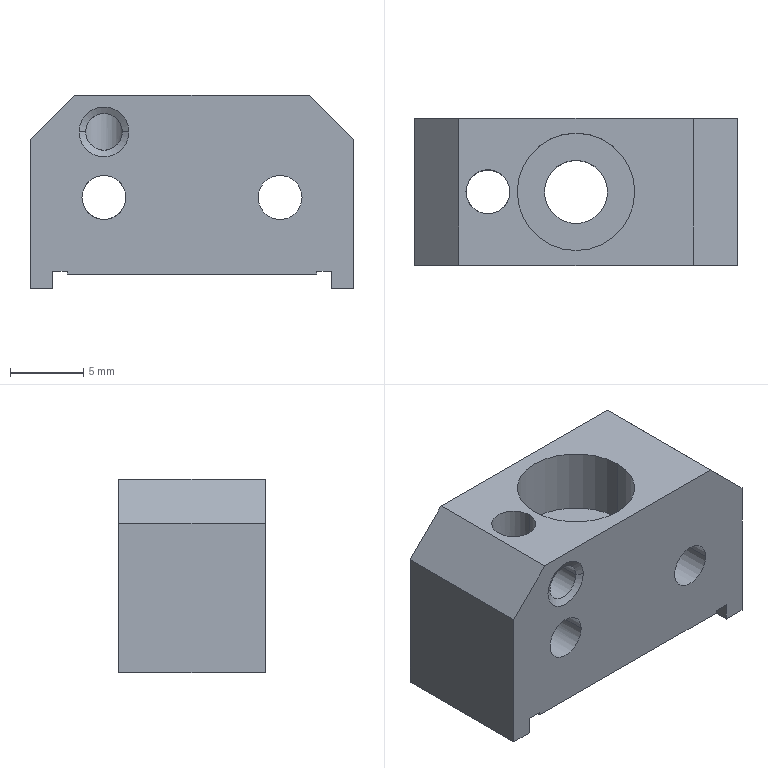Part | NX | 1 solid | 35 faces | box 22 x 10 x 13.2 mm | volume 2054 mm3 | plane 17 | cylinder 16 | cone 2 | commonest cylinder face diameters 3 x10 2.5 x2 4.3 x2 8 x2
STEP:
#1=CARTESIAN_POINT('',(9.5,5.,-6.6));
#2=VERTEX_POINT('',#1);
#3=CARTESIAN_POINT('',(9.5,-5.,-6.6));
#4=VERTEX_POINT('',#3);
#5=CARTESIAN_POINT('',(9.5,5.,-6.6));
#6=DIRECTION('',(0.,-1.,0.));
#7=VECTOR('',#6,1000.);
#8=LINE('',#5,#7);
#9=EDGE_CURVE('',#2,#4,#8,.T.);
#10=ORIENTED_EDGE('',*,*,#9,.F.);
#11=CARTESIAN_POINT('',(11.,5.,-6.6));
#12=VERTEX_POINT('',#11);
#13=CARTESIAN_POINT('',(0.,5.,-6.6));
#14=DIRECTION('',(-1.,0.,0.));
#15=VECTOR('',#14,1000.);
#16=LINE('',#13,#15);
#17=EDGE_CURVE('',#12,#2,#16,.T.);
#18=ORIENTED_EDGE('',*,*,#17,.F.);
#19=CARTESIAN_POINT('',(11.,-5.,-6.6));
#20=VERTEX_POINT('',#19);
#21=CARTESIAN_POINT('',(11.,5.,-6.6));
#22=DIRECTION('',(0.,-1.,0.));
#23=VECTOR('',#22,1000.);
#24=LINE('',#21,#23);
#25=EDGE_CURVE('',#12,#20,#24,.T.);
#26=ORIENTED_EDGE('',*,*,#25,.T.);
#27=CARTESIAN_POINT('',(0.,-5.,-6.6));
#28=DIRECTION('',(1.,0.,0.));
#29=VECTOR('',#28,1000.);
#30=LINE('',#27,#29);
#31=EDGE_CURVE('',#4,#20,#30,.T.);
#32=ORIENTED_EDGE('',*,*,#31,.F.);
#33=EDGE_LOOP('',(#10,#18,#26,#32));
#34=FACE_BOUND('',#33,.T.);
#35=CARTESIAN_POINT('',(0.,0.,-6.6));
#36=DIRECTION('',(0.,0.,1.));
#37=DIRECTION('',(1.,0.,0.));
#38=AXIS2_PLACEMENT_3D('',#35,#36,#37);
#39=PLANE('',#38);
#40=ADVANCED_FACE('',(#34),#39,.F.);
#41=CARTESIAN_POINT('',(9.5,5.,-5.4));
#42=VERTEX_POINT('',#41);
#43=CARTESIAN_POINT('',(9.5,5.,0.));
#44=DIRECTION('',(0.,0.,1.));
#45=VECTOR('',#44,1000.);
#46=LINE('',#43,#45);
#47=EDGE_CURVE('',#2,#42,#46,.T.);
#48=ORIENTED_EDGE('',*,*,#47,.F.);
#49=ORIENTED_EDGE('',*,*,#9,.T.);
#50=CARTESIAN_POINT('',(9.5,-5.,-5.4));
#51=VERTEX_POINT('',#50);
#52=CARTESIAN_POINT('',(9.5,-5.,0.));
#53=DIRECTION('',(0.,0.,-1.));
#54=VECTOR('',#53,1000.);
#55=LINE('',#52,#54);
#56=EDGE_CURVE('',#51,#4,#55,.T.);
#57=ORIENTED_EDGE('',*,*,#56,.F.);
#58=CARTESIAN_POINT('',(9.5,5.,-5.4));
#59=DIRECTION('',(0.,-1.,0.));
#60=VECTOR('',#59,1000.);
#61=LINE('',#58,#60);
#62=EDGE_CURVE('',#42,#51,#61,.T.);
#63=ORIENTED_EDGE('',*,*,#62,.F.);
#64=EDGE_LOOP('',(#48,#49,#57,#63));
#65=FACE_BOUND('',#64,.T.);
#66=CARTESIAN_POINT('',(9.5,-5.,-6.6));
#67=DIRECTION('',(1.,0.,0.));
#68=DIRECTION('',(0.,1.,0.));
#69=AXIS2_PLACEMENT_3D('',#66,#67,#68);
#70=PLANE('',#69);
#71=ADVANCED_FACE('',(#65),#70,.F.);
#72=CARTESIAN_POINT('',(-8.5,5.,-5.6));
#73=VERTEX_POINT('',#72);
#74=CARTESIAN_POINT('',(-8.5,5.,-5.4));
#75=VERTEX_POINT('',#74);
#76=CARTESIAN_POINT('',(-8.5,5.,0.));
#77=DIRECTION('',(0.,0.,1.));
#78=VECTOR('',#77,1000.);
#79=LINE('',#76,#78);
#80=EDGE_CURVE('',#73,#75,#79,.T.);
#81=ORIENTED_EDGE('',*,*,#80,.T.);
#82=CARTESIAN_POINT('',(-9.5,5.,-5.4));
#83=VERTEX_POINT('',#82);
#84=CARTESIAN_POINT('',(0.,5.,-5.4));
#85=DIRECTION('',(-1.,0.,0.));
#86=VECTOR('',#85,1000.);
#87=LINE('',#84,#86);
#88=EDGE_CURVE('',#75,#83,#87,.T.);
#89=ORIENTED_EDGE('',*,*,#88,.T.);
#90=CARTESIAN_POINT('',(-9.5,5.,-6.6));
#91=VERTEX_POINT('',#90);
#92=CARTESIAN_POINT('',(-9.5,5.,0.));
#93=DIRECTION('',(0.,0.,-1.));
#94=VECTOR('',#93,1000.);
#95=LINE('',#92,#94);
#96=EDGE_CURVE('',#83,#91,#95,.T.);
#97=ORIENTED_EDGE('',*,*,#96,.T.);
#98=CARTESIAN_POINT('',(-11.,5.,-6.6));
#99=VERTEX_POINT('',#98);
#100=CARTESIAN_POINT('',(0.,5.,-6.6));
#101=DIRECTION('',(-1.,0.,0.));
#102=VECTOR('',#101,1000.);
#103=LINE('',#100,#102);
#104=EDGE_CURVE('',#91,#99,#103,.T.);
#105=ORIENTED_EDGE('',*,*,#104,.T.);
#106=CARTESIAN_POINT('',(-11.,5.,3.6));
#107=VERTEX_POINT('',#106);
#108=CARTESIAN_POINT('',(-11.,5.,0.));
#109=DIRECTION('',(0.,0.,-1.));
#110=VECTOR('',#109,1000.);
#111=LINE('',#108,#110);
#112=EDGE_CURVE('',#107,#99,#111,.T.);
#113=ORIENTED_EDGE('',*,*,#112,.F.);
#114=CARTESIAN_POINT('',(-8.,5.,6.6));
#115=VERTEX_POINT('',#114);
#116=CARTESIAN_POINT('',(-14.6,5.,0.));
#117=DIRECTION('',(0.7071,0.,0.7071));
#118=VECTOR('',#117,1000.);
#119=LINE('',#116,#118);
#120=EDGE_CURVE('',#107,#115,#119,.T.);
#121=ORIENTED_EDGE('',*,*,#120,.T.);
#122=CARTESIAN_POINT('',(8.,5.,6.6));
#123=VERTEX_POINT('',#122);
#124=CARTESIAN_POINT('',(0.,5.,6.6));
#125=DIRECTION('',(-1.,0.,0.));
#126=VECTOR('',#125,1000.);
#127=LINE('',#124,#126);
#128=EDGE_CURVE('',#123,#115,#127,.T.);
#129=ORIENTED_EDGE('',*,*,#128,.F.);
#130=CARTESIAN_POINT('',(11.,5.,3.6));
#131=VERTEX_POINT('',#130);
#132=CARTESIAN_POINT('',(14.6,5.,0.));
#133=DIRECTION('',(0.7071,0.,-0.7071));
#134=VECTOR('',#133,1000.);
#135=LINE('',#132,#134);
#136=EDGE_CURVE('',#123,#131,#135,.T.);
#137=ORIENTED_EDGE('',*,*,#136,.T.);
#138=CARTESIAN_POINT('',(11.,5.,0.));
#139=DIRECTION('',(0.,0.,1.));
#140=VECTOR('',#139,1000.);
#141=LINE('',#138,#140);
#142=EDGE_CURVE('',#12,#131,#141,.T.);
#143=ORIENTED_EDGE('',*,*,#142,.F.);
#144=ORIENTED_EDGE('',*,*,#17,.T.);
#145=ORIENTED_EDGE('',*,*,#47,.T.);
#146=CARTESIAN_POINT('',(8.5,5.,-5.4));
#147=VERTEX_POINT('',#146);
#148=CARTESIAN_POINT('',(0.,5.,-5.4));
#149=DIRECTION('',(-1.,0.,0.));
#150=VECTOR('',#149,1000.);
#151=LINE('',#148,#150);
#152=EDGE_CURVE('',#42,#147,#151,.T.);
#153=ORIENTED_EDGE('',*,*,#152,.T.);
#154=CARTESIAN_POINT('',(8.5,5.,-5.6));
#155=VERTEX_POINT('',#154);
#156=CARTESIAN_POINT('',(8.5,5.,0.));
#157=DIRECTION('',(0.,0.,-1.));
#158=VECTOR('',#157,1000.);
#159=LINE('',#156,#158);
#160=EDGE_CURVE('',#147,#155,#159,.T.);
#161=ORIENTED_EDGE('',*,*,#160,.T.);
#162=CARTESIAN_POINT('',(0.,5.,-5.6));
#163=DIRECTION('',(-1.,0.,0.));
#164=VECTOR('',#163,1000.);
#165=LINE('',#162,#164);
#166=EDGE_CURVE('',#155,#73,#165,.T.);
#167=ORIENTED_EDGE('',*,*,#166,.T.);
#168=EDGE_LOOP('',(#81,#89,#97,#105,#113,#121,#129,#137,#143,#144,#145,#153,#161,#167));
#169=FACE_BOUND('',#168,.T.);
#170=CARTESIAN_POINT('',(-7.5,5.,-0.37));
#171=VERTEX_POINT('',#170);
#172=CARTESIAN_POINT('',(-4.5,5.,-0.37));
#173=VERTEX_POINT('',#172);
#174=CARTESIAN_POINT('',(-6.,5.,-0.37));
#175=DIRECTION('',(0.,1.,0.));
#176=DIRECTION('',(-1.,0.,0.));
#177=AXIS2_PLACEMENT_3D('',#174,#175,#176);
#178=CIRCLE('',#177,1.5);
#179=EDGE_CURVE('',#171,#173,#178,.T.);
#180=ORIENTED_EDGE('',*,*,#179,.F.);
#181=CARTESIAN_POINT('',(-6.,5.,-0.37));
#182=DIRECTION('',(0.,1.,0.));
#183=DIRECTION('',(-1.,0.,0.));
#184=AXIS2_PLACEMENT_3D('',#181,#182,#183);
#185=CIRCLE('',#184,1.5);
#186=EDGE_CURVE('',#173,#171,#185,.T.);
#187=ORIENTED_EDGE('',*,*,#186,.F.);
#188=EDGE_LOOP('',(#180,#187));
#189=FACE_BOUND('',#188,.T.);
#190=CARTESIAN_POINT('',(4.5,5.,-0.37));
#191=VERTEX_POINT('',#190);
#192=CARTESIAN_POINT('',(7.5,5.,-0.37));
#193=VERTEX_POINT('',#192);
#194=CARTESIAN_POINT('',(6.,5.,-0.37));
#195=DIRECTION('',(0.,1.,0.));
#196=DIRECTION('',(-1.,0.,0.));
#197=AXIS2_PLACEMENT_3D('',#194,#195,#196);
#198=CIRCLE('',#197,1.5);
#199=EDGE_CURVE('',#191,#193,#198,.T.);
#200=ORIENTED_EDGE('',*,*,#199,.F.);
#201=CARTESIAN_POINT('',(6.,5.,-0.37));
#202=DIRECTION('',(0.,1.,0.));
#203=DIRECTION('',(-1.,0.,0.));
#204=AXIS2_PLACEMENT_3D('',#201,#202,#203);
#205=CIRCLE('',#204,1.5);
#206=EDGE_CURVE('',#193,#191,#205,.T.);
#207=ORIENTED_EDGE('',*,*,#206,.F.);
#208=EDGE_LOOP('',(#200,#207));
#209=FACE_BOUND('',#208,.T.);
#210=CARTESIAN_POINT('',(11.,5.,-6.6));
#211=DIRECTION('',(0.,1.,0.));
#212=DIRECTION('',(1.,0.,0.));
#213=AXIS2_PLACEMENT_3D('',#210,#211,#212);
#214=PLANE('',#213);
#215=ADVANCED_FACE('',(#169,#189,#209),#214,.T.);
#216=CARTESIAN_POINT('',(-8.5,-5.,-5.4));
#217=VERTEX_POINT('',#216);
#218=CARTESIAN_POINT('',(-8.5,-5.,-5.6));
#219=VERTEX_POINT('',#218);
#220=CARTESIAN_POINT('',(-8.5,-5.,0.));
#221=DIRECTION('',(0.,0.,-1.));
#222=VECTOR('',#221,1000.);
#223=LINE('',#220,#222);
#224=EDGE_CURVE('',#217,#219,#223,.T.);
#225=ORIENTED_EDGE('',*,*,#224,.F.);
#226=CARTESIAN_POINT('',(-8.5,5.,-5.4));
#227=DIRECTION('',(0.,-1.,0.));
#228=VECTOR('',#227,1000.);
#229=LINE('',#226,#228);
#230=EDGE_CURVE('',#75,#217,#229,.T.);
#231=ORIENTED_EDGE('',*,*,#230,.F.);
#232=ORIENTED_EDGE('',*,*,#80,.F.);
#233=CARTESIAN_POINT('',(-8.5,0.,-5.6));
#234=DIRECTION('',(0.,-1.,0.));
#235=VECTOR('',#234,1000.);
#236=LINE('',#233,#235);
#237=EDGE_CURVE('',#73,#219,#236,.T.);
#238=ORIENTED_EDGE('',*,*,#237,.T.);
#239=EDGE_LOOP('',(#225,#231,#232,#238));
#240=FACE_BOUND('',#239,.T.);
#241=CARTESIAN_POINT('',(-8.5,-5.,-5.6));
#242=DIRECTION('',(1.,0.,0.));
#243=DIRECTION('',(0.,1.,0.));
#244=AXIS2_PLACEMENT_3D('',#241,#242,#243);
#245=PLANE('',#244);
#246=ADVANCED_FACE('',(#240),#245,.F.);
#247=ORIENTED_EDGE('',*,*,#224,.T.);
#248=CARTESIAN_POINT('',(8.5,-5.,-5.6));
#249=VERTEX_POINT('',#248);
#250=CARTESIAN_POINT('',(0.,-5.,-5.6));
#251=DIRECTION('',(1.,0.,0.));
#252=VECTOR('',#251,1000.);
#253=LINE('',#250,#252);
#254=EDGE_CURVE('',#219,#249,#253,.T.);
#255=ORIENTED_EDGE('',*,*,#254,.T.);
#256=CARTESIAN_POINT('',(8.5,-5.,-5.4));
#257=VERTEX_POINT('',#256);
#258=CARTESIAN_POINT('',(8.5,-5.,0.));
#259=DIRECTION('',(0.,0.,1.));
#260=VECTOR('',#259,1000.);
#261=LINE('',#258,#260);
#262=EDGE_CURVE('',#249,#257,#261,.T.);
#263=ORIENTED_EDGE('',*,*,#262,.T.);
#264=CARTESIAN_POINT('',(0.,-5.,-5.4));
#265=DIRECTION('',(1.,0.,0.));
#266=VECTOR('',#265,1000.);
#267=LINE('',#264,#266);
#268=EDGE_CURVE('',#257,#51,#267,.T.);
#269=ORIENTED_EDGE('',*,*,#268,.T.);
#270=ORIENTED_EDGE('',*,*,#56,.T.);
#271=ORIENTED_EDGE('',*,*,#31,.T.);
#272=CARTESIAN_POINT('',(11.,-5.,3.6));
#273=VERTEX_POINT('',#272);
#274=CARTESIAN_POINT('',(11.,-5.,0.));
#275=DIRECTION('',(0.,0.,-1.));
#276=VECTOR('',#275,1000.);
#277=LINE('',#274,#276);
#278=EDGE_CURVE('',#273,#20,#277,.T.);
#279=ORIENTED_EDGE('',*,*,#278,.F.);
#280=CARTESIAN_POINT('',(8.,-5.,6.6));
#281=VERTEX_POINT('',#280);
#282=CARTESIAN_POINT('',(14.6,-5.,0.));
#283=DIRECTION('',(-0.7071,0.,0.7071));
#284=VECTOR('',#283,1000.);
#285=LINE('',#282,#284);
#286=EDGE_CURVE('',#273,#281,#285,.T.);
#287=ORIENTED_EDGE('',*,*,#286,.T.);
#288=CARTESIAN_POINT('',(-8.,-5.,6.6));
#289=VERTEX_POINT('',#288);
#290=CARTESIAN_POINT('',(0.,-5.,6.6));
#291=DIRECTION('',(1.,0.,0.));
#292=VECTOR('',#291,1000.);
#293=LINE('',#290,#292);
#294=EDGE_CURVE('',#289,#281,#293,.T.);
#295=ORIENTED_EDGE('',*,*,#294,.F.);
#296=CARTESIAN_POINT('',(-11.,-5.,3.6));
#297=VERTEX_POINT('',#296);
#298=CARTESIAN_POINT('',(-14.6,-5.,0.));
#299=DIRECTION('',(-0.7071,0.,-0.7071));
#300=VECTOR('',#299,1000.);
#301=LINE('',#298,#300);
#302=EDGE_CURVE('',#289,#297,#301,.T.);
#303=ORIENTED_EDGE('',*,*,#302,.T.);
#304=CARTESIAN_POINT('',(-11.,-5.,-6.6));
#305=VERTEX_POINT('',#304);
#306=CARTESIAN_POINT('',(-11.,-5.,0.));
#307=DIRECTION('',(0.,0.,1.));
#308=VECTOR('',#307,1000.);
#309=LINE('',#306,#308);
#310=EDGE_CURVE('',#305,#297,#309,.T.);
#311=ORIENTED_EDGE('',*,*,#310,.F.);
#312=CARTESIAN_POINT('',(-9.5,-5.,-6.6));
#313=VERTEX_POINT('',#312);
#314=CARTESIAN_POINT('',(0.,-5.,-6.6));
#315=DIRECTION('',(1.,0.,0.));
#316=VECTOR('',#315,1000.);
#317=LINE('',#314,#316);
#318=EDGE_CURVE('',#305,#313,#317,.T.);
#319=ORIENTED_EDGE('',*,*,#318,.T.);
#320=CARTESIAN_POINT('',(-9.5,-5.,-5.4));
#321=VERTEX_POINT('',#320);
#322=CARTESIAN_POINT('',(-9.5,-5.,0.));
#323=DIRECTION('',(0.,0.,1.));
#324=VECTOR('',#323,1000.);
#325=LINE('',#322,#324);
#326=EDGE_CURVE('',#313,#321,#325,.T.);
#327=ORIENTED_EDGE('',*,*,#326,.T.);
#328=CARTESIAN_POINT('',(0.,-5.,-5.4));
#329=DIRECTION('',(1.,0.,0.));
#330=VECTOR('',#329,1000.);
#331=LINE('',#328,#330);
#332=EDGE_CURVE('',#321,#217,#331,.T.);
#333=ORIENTED_EDGE('',*,*,#332,.T.);
#334=EDGE_LOOP('',(#247,#255,#263,#269,#270,#271,#279,#287,#295,#303,#311,#319,#327,#333));
#335=FACE_BOUND('',#334,.T.);
#336=CARTESIAN_POINT('',(-4.5,-5.,-0.37));
#337=VERTEX_POINT('',#336);
#338=CARTESIAN_POINT('',(-7.5,-5.,-0.37));
#339=VERTEX_POINT('',#338);
#340=CARTESIAN_POINT('',(-6.,-5.,-0.37));
#341=DIRECTION('',(0.,1.,0.));
#342=DIRECTION('',(-1.,0.,0.));
#343=AXIS2_PLACEMENT_3D('',#340,#341,#342);
#344=CIRCLE('',#343,1.5);
#345=EDGE_CURVE('',#337,#339,#344,.T.);
#346=ORIENTED_EDGE('',*,*,#345,.T.);
#347=CARTESIAN_POINT('',(-6.,-5.,-0.37));
#348=DIRECTION('',(0.,1.,0.));
#349=DIRECTION('',(-1.,0.,0.));
#350=AXIS2_PLACEMENT_3D('',#347,#348,#349);
#351=CIRCLE('',#350,1.5);
#352=EDGE_CURVE('',#339,#337,#351,.T.);
#353=ORIENTED_EDGE('',*,*,#352,.T.);
#354=EDGE_LOOP('',(#346,#353));
#355=FACE_BOUND('',#354,.T.);
#356=CARTESIAN_POINT('',(-4.3,-5.,4.1));
#357=VERTEX_POINT('',#356);
#358=CARTESIAN_POINT('',(-7.7,-5.,4.1));
#359=VERTEX_POINT('',#358);
#360=CARTESIAN_POINT('',(-6.,-5.,4.1));
#361=DIRECTION('',(0.,-1.,0.));
#362=DIRECTION('',(-1.,0.,0.));
#363=AXIS2_PLACEMENT_3D('',#360,#361,#362);
#364=CIRCLE('',#363,1.7);
#365=EDGE_CURVE('',#357,#359,#364,.T.);
#366=ORIENTED_EDGE('',*,*,#365,.F.);
#367=CARTESIAN_POINT('',(-6.,-5.,4.1));
#368=DIRECTION('',(0.,-1.,0.));
#369=DIRECTION('',(-1.,0.,0.));
#370=AXIS2_PLACEMENT_3D('',#367,#368,#369);
#371=CIRCLE('',#370,1.7);
#372=EDGE_CURVE('',#359,#357,#371,.T.);
#373=ORIENTED_EDGE('',*,*,#372,.F.);
#374=EDGE_LOOP('',(#366,#373));
#375=FACE_BOUND('',#374,.T.);
#376=CARTESIAN_POINT('',(7.5,-5.,-0.37));
#377=VERTEX_POINT('',#376);
#378=CARTESIAN_POINT('',(4.5,-5.,-0.37));
#379=VERTEX_POINT('',#378);
#380=CARTESIAN_POINT('',(6.,-5.,-0.37));
#381=DIRECTION('',(0.,1.,0.));
#382=DIRECTION('',(-1.,0.,0.));
#383=AXIS2_PLACEMENT_3D('',#380,#381,#382);
#384=CIRCLE('',#383,1.5);
#385=EDGE_CURVE('',#377,#379,#384,.T.);
#386=ORIENTED_EDGE('',*,*,#385,.T.);
#387=CARTESIAN_POINT('',(6.,-5.,-0.37));
#388=DIRECTION('',(0.,1.,0.));
#389=DIRECTION('',(-1.,0.,0.));
#390=AXIS2_PLACEMENT_3D('',#387,#388,#389);
#391=CIRCLE('',#390,1.5);
#392=EDGE_CURVE('',#379,#377,#391,.T.);
#393=ORIENTED_EDGE('',*,*,#392,.T.);
#394=EDGE_LOOP('',(#386,#393));
#395=FACE_BOUND('',#394,.T.);
#396=CARTESIAN_POINT('',(-11.,-5.,-6.6));
#397=DIRECTION('',(0.,-1.,0.));
#398=DIRECTION('',(0.,0.,-1.));
#399=AXIS2_PLACEMENT_3D('',#396,#397,#398);
#400=PLANE('',#399);
#401=ADVANCED_FACE('',(#335,#355,#375,#395),#400,.T.);
#402=ORIENTED_EDGE('',*,*,#332,.F.);
#403=CARTESIAN_POINT('',(-9.5,5.,-5.4));
#404=DIRECTION('',(0.,-1.,0.));
#405=VECTOR('',#404,1000.);
#406=LINE('',#403,#405);
#407=EDGE_CURVE('',#83,#321,#406,.T.);
#408=ORIENTED_EDGE('',*,*,#407,.F.);
#409=ORIENTED_EDGE('',*,*,#88,.F.);
#410=ORIENTED_EDGE('',*,*,#230,.T.);
#411=EDGE_LOOP('',(#402,#408,#409,#410));
#412=FACE_BOUND('',#411,.T.);
#413=CARTESIAN_POINT('',(-8.5,-5.,-5.4));
#414=DIRECTION('',(0.,0.,1.));
#415=DIRECTION('',(1.,0.,0.));
#416=AXIS2_PLACEMENT_3D('',#413,#414,#415);
#417=PLANE('',#416);
#418=ADVANCED_FACE('',(#412),#417,.F.);
#419=ORIENTED_EDGE('',*,*,#326,.F.);
#420=CARTESIAN_POINT('',(-9.5,5.,-6.6));
#421=DIRECTION('',(0.,-1.,0.));
#422=VECTOR('',#421,1000.);
#423=LINE('',#420,#422);
#424=EDGE_CURVE('',#91,#313,#423,.T.);
#425=ORIENTED_EDGE('',*,*,#424,.F.);
#426=ORIENTED_EDGE('',*,*,#96,.F.);
#427=ORIENTED_EDGE('',*,*,#407,.T.);
#428=EDGE_LOOP('',(#419,#425,#426,#427));
#429=FACE_BOUND('',#428,.T.);
#430=CARTESIAN_POINT('',(-9.5,-5.,-5.6));
#431=DIRECTION('',(-1.,0.,0.));
#432=DIRECTION('',(0.,0.,1.));
#433=AXIS2_PLACEMENT_3D('',#430,#431,#432);
#434=PLANE('',#433);
#435=ADVANCED_FACE('',(#429),#434,.F.);
#436=ORIENTED_EDGE('',*,*,#424,.T.);
#437=ORIENTED_EDGE('',*,*,#318,.F.);
#438=CARTESIAN_POINT('',(-11.,-5.,-6.6));
#439=DIRECTION('',(0.,1.,0.));
#440=VECTOR('',#439,1000.);
#441=LINE('',#438,#440);
#442=EDGE_CURVE('',#305,#99,#441,.T.);
#443=ORIENTED_EDGE('',*,*,#442,.T.);
#444=ORIENTED_EDGE('',*,*,#104,.F.);
#445=EDGE_LOOP('',(#436,#437,#443,#444));
#446=FACE_BOUND('',#445,.T.);
#447=CARTESIAN_POINT('',(0.,0.,-6.6));
#448=DIRECTION('',(0.,0.,1.));
#449=DIRECTION('',(1.,0.,0.));
#450=AXIS2_PLACEMENT_3D('',#447,#448,#449);
#451=PLANE('',#450);
#452=ADVANCED_FACE('',(#446),#451,.F.);
#453=CARTESIAN_POINT('',(-11.,0.,3.6));
#454=DIRECTION('',(0.,1.,0.));
#455=VECTOR('',#454,1000.);
#456=LINE('',#453,#455);
#457=EDGE_CURVE('',#297,#107,#456,.T.);
#458=ORIENTED_EDGE('',*,*,#457,.T.);
#459=ORIENTED_EDGE('',*,*,#112,.T.);
#460=ORIENTED_EDGE('',*,*,#442,.F.);
#461=ORIENTED_EDGE('',*,*,#310,.T.);
#462=EDGE_LOOP('',(#458,#459,#460,#461));
#463=FACE_BOUND('',#462,.T.);
#464=CARTESIAN_POINT('',(-11.,5.,-6.6));
#465=DIRECTION('',(-1.,0.,0.));
#466=DIRECTION('',(0.,0.,1.));
#467=AXIS2_PLACEMENT_3D('',#464,#465,#466);
#468=PLANE('',#467);
#469=ADVANCED_FACE('',(#463),#468,.T.);
#470=CARTESIAN_POINT('',(8.,0.,6.6));
#471=DIRECTION('',(0.,1.,0.));
#472=VECTOR('',#471,1000.);
#473=LINE('',#470,#472);
#474=EDGE_CURVE('',#281,#123,#473,.T.);
#475=ORIENTED_EDGE('',*,*,#474,.T.);
#476=ORIENTED_EDGE('',*,*,#128,.T.);
#477=CARTESIAN_POINT('',(-8.,0.,6.6));
#478=DIRECTION('',(0.,-1.,0.));
#479=VECTOR('',#478,1000.);
#480=LINE('',#477,#479);
#481=EDGE_CURVE('',#115,#289,#480,.T.);
#482=ORIENTED_EDGE('',*,*,#481,.T.);
#483=ORIENTED_EDGE('',*,*,#294,.T.);
#484=EDGE_LOOP('',(#475,#476,#482,#483));
#485=FACE_BOUND('',#484,.T.);
#486=CARTESIAN_POINT('',(-4.,0.,6.6));
#487=VERTEX_POINT('',#486);
#488=CARTESIAN_POINT('',(4.,0.,6.6));
#489=VERTEX_POINT('',#488);
#490=CARTESIAN_POINT('',(0.,0.,6.6));
#491=DIRECTION('',(0.,0.,1.));
#492=DIRECTION('',(1.,0.,0.));
#493=AXIS2_PLACEMENT_3D('',#490,#491,#492);
#494=CIRCLE('',#493,4.);
#495=EDGE_CURVE('',#487,#489,#494,.T.);
#496=ORIENTED_EDGE('',*,*,#495,.F.);
#497=CARTESIAN_POINT('',(0.,0.,6.6));
#498=DIRECTION('',(0.,0.,1.));
#499=DIRECTION('',(1.,0.,0.));
#500=AXIS2_PLACEMENT_3D('',#497,#498,#499);
#501=CIRCLE('',#500,4.);
#502=EDGE_CURVE('',#489,#487,#501,.T.);
#503=ORIENTED_EDGE('',*,*,#502,.F.);
#504=EDGE_LOOP('',(#496,#503));
#505=FACE_BOUND('',#504,.T.);
#506=CARTESIAN_POINT('',(-7.5,0.,6.6));
#507=VERTEX_POINT('',#506);
#508=CARTESIAN_POINT('',(-4.5,0.,6.6));
#509=VERTEX_POINT('',#508);
#510=CARTESIAN_POINT('',(-6.,0.,6.6));
#511=DIRECTION('',(0.,0.,-1.));
#512=DIRECTION('',(-1.,0.,0.));
#513=AXIS2_PLACEMENT_3D('',#510,#511,#512);
#514=CIRCLE('',#513,1.5);
#515=EDGE_CURVE('',#507,#509,#514,.T.);
#516=ORIENTED_EDGE('',*,*,#515,.T.);
#517=CARTESIAN_POINT('',(-6.,0.,6.6));
#518=DIRECTION('',(0.,0.,-1.));
#519=DIRECTION('',(-1.,0.,0.));
#520=AXIS2_PLACEMENT_3D('',#517,#518,#519);
#521=CIRCLE('',#520,1.5);
#522=EDGE_CURVE('',#509,#507,#521,.T.);
#523=ORIENTED_EDGE('',*,*,#522,.T.);
#524=EDGE_LOOP('',(#516,#523));
#525=FACE_BOUND('',#524,.T.);
#526=CARTESIAN_POINT('',(0.,0.,6.6));
#527=DIRECTION('',(0.,0.,1.));
#528=DIRECTION('',(1.,0.,0.));
#529=AXIS2_PLACEMENT_3D('',#526,#527,#528);
#530=PLANE('',#529);
#531=ADVANCED_FACE('',(#485,#505,#525),#530,.T.);
#532=ORIENTED_EDGE('',*,*,#25,.F.);
#533=ORIENTED_EDGE('',*,*,#142,.T.);
#534=CARTESIAN_POINT('',(11.,0.,3.6));
#535=DIRECTION('',(0.,-1.,0.));
#536=VECTOR('',#535,1000.);
#537=LINE('',#534,#536);
#538=EDGE_CURVE('',#131,#273,#537,.T.);
#539=ORIENTED_EDGE('',*,*,#538,.T.);
#540=ORIENTED_EDGE('',*,*,#278,.T.);
#541=EDGE_LOOP('',(#532,#533,#539,#540));
#542=FACE_BOUND('',#541,.T.);
#543=CARTESIAN_POINT('',(11.,-5.,-6.6));
#544=DIRECTION('',(1.,0.,0.));
#545=DIRECTION('',(0.,1.,0.));
#546=AXIS2_PLACEMENT_3D('',#543,#544,#545);
#547=PLANE('',#546);
#548=ADVANCED_FACE('',(#542),#547,.T.);
#549=ORIENTED_EDGE('',*,*,#495,.T.);
#550=CARTESIAN_POINT('',(4.,0.,2.1));
#551=VERTEX_POINT('',#550);
#552=CARTESIAN_POINT('',(4.,0.,-8.646));
#553=DIRECTION('',(0.,0.,1.));
#554=VECTOR('',#553,1000.);
#555=LINE('',#552,#554);
#556=EDGE_CURVE('',#551,#489,#555,.T.);
#557=ORIENTED_EDGE('',*,*,#556,.F.);
#558=CARTESIAN_POINT('',(-4.,0.,2.1));
#559=VERTEX_POINT('',#558);
#560=CARTESIAN_POINT('',(0.,0.,2.1));
#561=DIRECTION('',(0.,0.,-1.));
#562=DIRECTION('',(-1.,0.,0.));
#563=AXIS2_PLACEMENT_3D('',#560,#561,#562);
#564=CIRCLE('',#563,4.);
#565=EDGE_CURVE('',#551,#559,#564,.T.);
#566=ORIENTED_EDGE('',*,*,#565,.T.);
#567=CARTESIAN_POINT('',(-4.,0.,-8.646));
#568=DIRECTION('',(0.,0.,1.));
#569=VECTOR('',#568,1000.);
#570=LINE('',#567,#569);
#571=EDGE_CURVE('',#559,#487,#570,.T.);
#572=ORIENTED_EDGE('',*,*,#571,.T.);
#573=EDGE_LOOP('',(#549,#557,#566,#572));
#574=FACE_BOUND('',#573,.T.);
#575=CARTESIAN_POINT('',(0.,0.,-8.646));
#576=DIRECTION('',(0.,0.,1.));
#577=DIRECTION('',(-1.,0.,0.));
#578=AXIS2_PLACEMENT_3D('',#575,#576,#577);
#579=CYLINDRICAL_SURFACE('',#578,4.);
#580=ADVANCED_FACE('',(#574),#579,.F.);
#581=CARTESIAN_POINT('',(-4.5,0.,-0.37));
#582=VERTEX_POINT('',#581);
#583=CARTESIAN_POINT('',(-7.5,0.,-0.37));
#584=VERTEX_POINT('',#583);
#585=CARTESIAN_POINT('',(-4.5,0.,-0.37));
#586=CARTESIAN_POINT('',(-4.5,-3.,-3.37));
#587=CARTESIAN_POINT('',(-7.5,-3.,-3.37));
#588=CARTESIAN_POINT('',(-7.5,0.,-0.37));
#589=(BOUNDED_CURVE()B_SPLINE_CURVE(3,(#585,#586,#587,#588),.UNSPECIFIED.,.F.,.F.)B_SPLINE_CURVE_WITH_KNOTS((4,4),(4.712,7.854),.UNSPECIFIED.)CURVE()GEOMETRIC_REPRESENTATION_ITEM()RATIONAL_B_SPLINE_CURVE((1.,0.3333,0.3333,1.))REPRESENTATION_ITEM(''));
#590=EDGE_CURVE('',#582,#584,#589,.T.);
#591=ORIENTED_EDGE('',*,*,#590,.T.);
#592=CARTESIAN_POINT('',(-7.5,-5.,-0.37));
#593=DIRECTION('',(0.,1.,0.));
#594=VECTOR('',#593,1000.);
#595=LINE('',#592,#594);
#596=EDGE_CURVE('',#584,#339,#595,.F.);
#597=ORIENTED_EDGE('',*,*,#596,.T.);
#598=ORIENTED_EDGE('',*,*,#345,.F.);
#599=CARTESIAN_POINT('',(-4.5,-5.,-0.37));
#600=DIRECTION('',(0.,1.,0.));
#601=VECTOR('',#600,1000.);
#602=LINE('',#599,#601);
#603=EDGE_CURVE('',#582,#337,#602,.F.);
#604=ORIENTED_EDGE('',*,*,#603,.F.);
#605=EDGE_LOOP('',(#591,#597,#598,#604));
#606=FACE_BOUND('',#605,.T.);
#607=CARTESIAN_POINT('',(-6.,-5.,-0.37));
#608=DIRECTION('',(0.,1.,0.));
#609=DIRECTION('',(-1.,0.,0.));
#610=AXIS2_PLACEMENT_3D('',#607,#608,#609);
#611=CYLINDRICAL_SURFACE('',#610,1.5);
#612=ADVANCED_FACE('',(#606),#611,.F.);
#613=CARTESIAN_POINT('',(0.,0.,2.1));
#614=DIRECTION('',(0.,0.,-1.));
#615=DIRECTION('',(-1.,0.,0.));
#616=AXIS2_PLACEMENT_3D('',#613,#614,#615);
#617=CIRCLE('',#616,4.);
#618=EDGE_CURVE('',#559,#551,#617,.T.);
#619=ORIENTED_EDGE('',*,*,#618,.F.);
#620=ORIENTED_EDGE('',*,*,#565,.F.);
#621=EDGE_LOOP('',(#619,#620));
#622=FACE_BOUND('',#621,.T.);
#623=CARTESIAN_POINT('',(2.15,0.,2.1));
#624=VERTEX_POINT('',#623);
#625=CARTESIAN_POINT('',(-2.15,0.,2.1));
#626=VERTEX_POINT('',#625);
#627=CARTESIAN_POINT('',(0.,0.,2.1));
#628=DIRECTION('',(0.,0.,1.));
#629=DIRECTION('',(-1.,0.,0.));
#630=AXIS2_PLACEMENT_3D('',#627,#628,#629);
#631=CIRCLE('',#630,2.15);
#632=EDGE_CURVE('',#624,#626,#631,.T.);
#633=ORIENTED_EDGE('',*,*,#632,.F.);
#634=CARTESIAN_POINT('',(0.,0.,2.1));
#635=DIRECTION('',(0.,0.,1.));
#636=DIRECTION('',(-1.,0.,0.));
#637=AXIS2_PLACEMENT_3D('',#634,#635,#636);
#638=CIRCLE('',#637,2.15);
#639=EDGE_CURVE('',#626,#624,#638,.T.);
#640=ORIENTED_EDGE('',*,*,#639,.F.);
#641=EDGE_LOOP('',(#633,#640));
#642=FACE_BOUND('',#641,.T.);
#643=CARTESIAN_POINT('',(0.,0.,2.1));
#644=DIRECTION('',(0.,0.,1.));
#645=DIRECTION('',(1.,0.,0.));
#646=AXIS2_PLACEMENT_3D('',#643,#644,#645);
#647=PLANE('',#646);
#648=ADVANCED_FACE('',(#622,#642),#647,.T.);
#649=ORIENTED_EDGE('',*,*,#632,.T.);
#650=CARTESIAN_POINT('',(-2.15,0.,-5.6));
#651=VERTEX_POINT('',#650);
#652=CARTESIAN_POINT('',(-2.15,0.,-8.646));
#653=DIRECTION('',(0.,0.,1.));
#654=VECTOR('',#653,1000.);
#655=LINE('',#652,#654);
#656=EDGE_CURVE('',#626,#651,#655,.F.);
#657=ORIENTED_EDGE('',*,*,#656,.T.);
#658=CARTESIAN_POINT('',(2.15,0.,-5.6));
#659=VERTEX_POINT('',#658);
#660=CARTESIAN_POINT('',(0.,0.,-5.6));
#661=DIRECTION('',(0.,0.,1.));
#662=DIRECTION('',(-1.,0.,0.));
#663=AXIS2_PLACEMENT_3D('',#660,#661,#662);
#664=CIRCLE('',#663,2.15);
#665=EDGE_CURVE('',#659,#651,#664,.T.);
#666=ORIENTED_EDGE('',*,*,#665,.F.);
#667=CARTESIAN_POINT('',(2.15,0.,-8.646));
#668=DIRECTION('',(0.,0.,1.));
#669=VECTOR('',#668,1000.);
#670=LINE('',#667,#669);
#671=EDGE_CURVE('',#624,#659,#670,.F.);
#672=ORIENTED_EDGE('',*,*,#671,.F.);
#673=EDGE_LOOP('',(#649,#657,#666,#672));
#674=FACE_BOUND('',#673,.T.);
#675=CARTESIAN_POINT('',(0.,0.,-8.646));
#676=DIRECTION('',(0.,0.,1.));
#677=DIRECTION('',(-1.,0.,0.));
#678=AXIS2_PLACEMENT_3D('',#675,#676,#677);
#679=CYLINDRICAL_SURFACE('',#678,2.15);
#680=ADVANCED_FACE('',(#674),#679,.F.);
#681=ORIENTED_EDGE('',*,*,#237,.F.);
#682=ORIENTED_EDGE('',*,*,#166,.F.);
#683=CARTESIAN_POINT('',(8.5,0.,-5.6));
#684=DIRECTION('',(0.,1.,0.));
#685=VECTOR('',#684,1000.);
#686=LINE('',#683,#685);
#687=EDGE_CURVE('',#249,#155,#686,.T.);
#688=ORIENTED_EDGE('',*,*,#687,.F.);
#689=ORIENTED_EDGE('',*,*,#254,.F.);
#690=EDGE_LOOP('',(#681,#682,#688,#689));
#691=FACE_BOUND('',#690,.T.);
#692=ORIENTED_EDGE('',*,*,#665,.T.);
#693=CARTESIAN_POINT('',(0.,0.,-5.6));
#694=DIRECTION('',(0.,0.,1.));
#695=DIRECTION('',(-1.,0.,0.));
#696=AXIS2_PLACEMENT_3D('',#693,#694,#695);
#697=CIRCLE('',#696,2.15);
#698=EDGE_CURVE('',#651,#659,#697,.T.);
#699=ORIENTED_EDGE('',*,*,#698,.T.);
#700=EDGE_LOOP('',(#692,#699));
#701=FACE_BOUND('',#700,.T.);
#702=CARTESIAN_POINT('',(-7.5,0.,-5.6));
#703=VERTEX_POINT('',#702);
#704=CARTESIAN_POINT('',(-4.5,0.,-5.6));
#705=VERTEX_POINT('',#704);
#706=CARTESIAN_POINT('',(-6.,0.,-5.6));
#707=DIRECTION('',(0.,0.,-1.));
#708=DIRECTION('',(-1.,0.,0.));
#709=AXIS2_PLACEMENT_3D('',#706,#707,#708);
#710=CIRCLE('',#709,1.5);
#711=EDGE_CURVE('',#703,#705,#710,.T.);
#712=ORIENTED_EDGE('',*,*,#711,.F.);
#713=CARTESIAN_POINT('',(-6.,0.,-5.6));
#714=DIRECTION('',(0.,0.,-1.));
#715=DIRECTION('',(-1.,0.,0.));
#716=AXIS2_PLACEMENT_3D('',#713,#714,#715);
#717=CIRCLE('',#716,1.5);
#718=EDGE_CURVE('',#705,#703,#717,.T.);
#719=ORIENTED_EDGE('',*,*,#718,.F.);
#720=EDGE_LOOP('',(#712,#719));
#721=FACE_BOUND('',#720,.T.);
#722=CARTESIAN_POINT('',(9.5,-5.,-5.6));
#723=DIRECTION('',(0.,0.,1.));
#724=DIRECTION('',(1.,0.,0.));
#725=AXIS2_PLACEMENT_3D('',#722,#723,#724);
#726=PLANE('',#725);
#727=ADVANCED_FACE('',(#691,#701,#721),#726,.F.);
#728=ORIENTED_EDGE('',*,*,#262,.F.);
#729=ORIENTED_EDGE('',*,*,#687,.T.);
#730=ORIENTED_EDGE('',*,*,#160,.F.);
#731=CARTESIAN_POINT('',(8.5,5.,-5.4));
#732=DIRECTION('',(0.,-1.,0.));
#733=VECTOR('',#732,1000.);
#734=LINE('',#731,#733);
#735=EDGE_CURVE('',#147,#257,#734,.T.);
#736=ORIENTED_EDGE('',*,*,#735,.T.);
#737=EDGE_LOOP('',(#728,#729,#730,#736));
#738=FACE_BOUND('',#737,.T.);
#739=CARTESIAN_POINT('',(8.5,-5.,-5.4));
#740=DIRECTION('',(-1.,0.,0.));
#741=DIRECTION('',(0.,0.,1.));
#742=AXIS2_PLACEMENT_3D('',#739,#740,#741);
#743=PLANE('',#742);
#744=ADVANCED_FACE('',(#738),#743,.F.);
#745=ORIENTED_EDGE('',*,*,#268,.F.);
#746=ORIENTED_EDGE('',*,*,#735,.F.);
#747=ORIENTED_EDGE('',*,*,#152,.F.);
#748=ORIENTED_EDGE('',*,*,#62,.T.);
#749=EDGE_LOOP('',(#745,#746,#747,#748));
#750=FACE_BOUND('',#749,.T.);
#751=CARTESIAN_POINT('',(9.5,-5.,-5.4));
#752=DIRECTION('',(0.,0.,1.));
#753=DIRECTION('',(1.,0.,0.));
#754=AXIS2_PLACEMENT_3D('',#751,#752,#753);
#755=PLANE('',#754);
#756=ADVANCED_FACE('',(#750),#755,.F.);
#757=ORIENTED_EDGE('',*,*,#385,.F.);
#758=CARTESIAN_POINT('',(7.5,-5.,-0.37));
#759=DIRECTION('',(0.,1.,0.));
#760=VECTOR('',#759,1000.);
#761=LINE('',#758,#760);
#762=EDGE_CURVE('',#377,#193,#761,.T.);
#763=ORIENTED_EDGE('',*,*,#762,.T.);
#764=ORIENTED_EDGE('',*,*,#206,.T.);
#765=CARTESIAN_POINT('',(4.5,-5.,-0.37));
#766=DIRECTION('',(0.,1.,0.));
#767=VECTOR('',#766,1000.);
#768=LINE('',#765,#767);
#769=EDGE_CURVE('',#379,#191,#768,.T.);
#770=ORIENTED_EDGE('',*,*,#769,.F.);
#771=EDGE_LOOP('',(#757,#763,#764,#770));
#772=FACE_BOUND('',#771,.T.);
#773=CARTESIAN_POINT('',(6.,-5.,-0.37));
#774=DIRECTION('',(0.,1.,0.));
#775=DIRECTION('',(-1.,0.,0.));
#776=AXIS2_PLACEMENT_3D('',#773,#774,#775);
#777=CYLINDRICAL_SURFACE('',#776,1.5);
#778=ADVANCED_FACE('',(#772),#777,.F.);
#779=CARTESIAN_POINT('',(-7.5,0.,-0.37));
#780=CARTESIAN_POINT('',(-7.5,3.,-3.37));
#781=CARTESIAN_POINT('',(-4.5,3.,-3.37));
#782=CARTESIAN_POINT('',(-4.5,0.,-0.37));
#783=(BOUNDED_CURVE()B_SPLINE_CURVE(3,(#779,#780,#781,#782),.UNSPECIFIED.,.F.,.F.)B_SPLINE_CURVE_WITH_KNOTS((4,4),(4.712,7.854),.UNSPECIFIED.)CURVE()GEOMETRIC_REPRESENTATION_ITEM()RATIONAL_B_SPLINE_CURVE((1.,0.3333,0.3333,1.))REPRESENTATION_ITEM(''));
#784=EDGE_CURVE('',#584,#582,#783,.T.);
#785=ORIENTED_EDGE('',*,*,#784,.F.);
#786=CARTESIAN_POINT('',(-7.5,0.,6.6));
#787=DIRECTION('',(0.,0.,-1.));
#788=VECTOR('',#787,1000.);
#789=LINE('',#786,#788);
#790=EDGE_CURVE('',#703,#584,#789,.F.);
#791=ORIENTED_EDGE('',*,*,#790,.F.);
#792=ORIENTED_EDGE('',*,*,#711,.T.);
#793=CARTESIAN_POINT('',(-4.5,0.,6.6));
#794=DIRECTION('',(0.,0.,-1.));
#795=VECTOR('',#794,1000.);
#796=LINE('',#793,#795);
#797=EDGE_CURVE('',#705,#582,#796,.F.);
#798=ORIENTED_EDGE('',*,*,#797,.T.);
#799=EDGE_LOOP('',(#785,#791,#792,#798));
#800=FACE_BOUND('',#799,.T.);
#801=CARTESIAN_POINT('',(-6.,0.,6.6));
#802=DIRECTION('',(0.,0.,-1.));
#803=DIRECTION('',(-1.,0.,0.));
#804=AXIS2_PLACEMENT_3D('',#801,#802,#803);
#805=CYLINDRICAL_SURFACE('',#804,1.5);
#806=ADVANCED_FACE('',(#800),#805,.F.);
#807=ORIENTED_EDGE('',*,*,#784,.T.);
#808=CARTESIAN_POINT('',(-4.5,-5.,-0.37));
#809=DIRECTION('',(0.,1.,0.));
#810=VECTOR('',#809,1000.);
#811=LINE('',#808,#810);
#812=EDGE_CURVE('',#582,#173,#811,.T.);
#813=ORIENTED_EDGE('',*,*,#812,.T.);
#814=ORIENTED_EDGE('',*,*,#186,.T.);
#815=CARTESIAN_POINT('',(-7.5,-5.,-0.37));
#816=DIRECTION('',(0.,1.,0.));
#817=VECTOR('',#816,1000.);
#818=LINE('',#815,#817);
#819=EDGE_CURVE('',#584,#171,#818,.T.);
#820=ORIENTED_EDGE('',*,*,#819,.F.);
#821=EDGE_LOOP('',(#807,#813,#814,#820));
#822=FACE_BOUND('',#821,.T.);
#823=CARTESIAN_POINT('',(-6.,-5.,-0.37));
#824=DIRECTION('',(0.,1.,0.));
#825=DIRECTION('',(-1.,0.,0.));
#826=AXIS2_PLACEMENT_3D('',#823,#824,#825);
#827=CYLINDRICAL_SURFACE('',#826,1.5);
#828=ADVANCED_FACE('',(#822),#827,.F.);
#829=CARTESIAN_POINT('',(-7.5,0.,-0.37));
#830=CARTESIAN_POINT('',(-7.5,3.,2.63));
#831=CARTESIAN_POINT('',(-4.5,3.,2.63));
#832=CARTESIAN_POINT('',(-4.5,0.,-0.37));
#833=(BOUNDED_CURVE()B_SPLINE_CURVE(3,(#829,#830,#831,#832),.UNSPECIFIED.,.F.,.F.)B_SPLINE_CURVE_WITH_KNOTS((4,4),(1.571,4.712),.UNSPECIFIED.)CURVE()GEOMETRIC_REPRESENTATION_ITEM()RATIONAL_B_SPLINE_CURVE((1.,0.3333,0.3333,1.))REPRESENTATION_ITEM(''));
#834=EDGE_CURVE('',#584,#582,#833,.T.);
#835=ORIENTED_EDGE('',*,*,#834,.T.);
#836=CARTESIAN_POINT('',(-4.5,0.,6.6));
#837=DIRECTION('',(0.,0.,-1.));
#838=VECTOR('',#837,1000.);
#839=LINE('',#836,#838);
#840=EDGE_CURVE('',#582,#509,#839,.F.);
#841=ORIENTED_EDGE('',*,*,#840,.T.);
#842=ORIENTED_EDGE('',*,*,#515,.F.);
#843=CARTESIAN_POINT('',(-7.5,0.,6.6));
#844=DIRECTION('',(0.,0.,-1.));
#845=VECTOR('',#844,1000.);
#846=LINE('',#843,#845);
#847=EDGE_CURVE('',#584,#507,#846,.F.);
#848=ORIENTED_EDGE('',*,*,#847,.F.);
#849=EDGE_LOOP('',(#835,#841,#842,#848));
#850=FACE_BOUND('',#849,.T.);
#851=CARTESIAN_POINT('',(-6.,0.,6.6));
#852=DIRECTION('',(0.,0.,-1.));
#853=DIRECTION('',(-1.,0.,0.));
#854=AXIS2_PLACEMENT_3D('',#851,#852,#853);
#855=CYLINDRICAL_SURFACE('',#854,1.5);
#856=ADVANCED_FACE('',(#850),#855,.F.);
#857=CARTESIAN_POINT('',(-4.75,-0.8292,4.1));
#858=VERTEX_POINT('',#857);
#859=CARTESIAN_POINT('',(-7.25,-0.8292,4.1));
#860=VERTEX_POINT('',#859);
#861=CARTESIAN_POINT('',(-4.75,-0.8292,4.1));
#862=CARTESIAN_POINT('',(-4.75,-0.8292,3.934));
#863=CARTESIAN_POINT('',(-4.828,-0.9361,3.646));
#864=CARTESIAN_POINT('',(-4.907,-1.037,3.47));
#865=CARTESIAN_POINT('',(-5.078,-1.185,3.252));
#866=CARTESIAN_POINT('',(-5.098,-1.2,3.233));
#867=CARTESIAN_POINT('',(-5.321,-1.346,3.036));
#868=CARTESIAN_POINT('',(-5.543,-1.438,2.927));
#869=CARTESIAN_POINT('',(-6.,-1.542,2.799));
#870=CARTESIAN_POINT('',(-6.457,-1.438,2.926));
#871=CARTESIAN_POINT('',(-6.68,-1.345,3.037));
#872=CARTESIAN_POINT('',(-6.9,-1.202,3.23));
#873=CARTESIAN_POINT('',(-6.925,-1.182,3.256));
#874=CARTESIAN_POINT('',(-7.09,-1.039,3.467));
#875=CARTESIAN_POINT('',(-7.174,-0.9344,3.648));
#876=CARTESIAN_POINT('',(-7.25,-0.8292,3.934));
#877=CARTESIAN_POINT('',(-7.25,-0.8292,4.1));
#878=B_SPLINE_CURVE_WITH_KNOTS('',3,(#861,#862,#863,#864,#865,#866,#867,#868,#869,#870,#871,#872,#873,#874,#875,#876,#877),.UNSPECIFIED.,.F.,.F.,(4,1,1,1,1,1,1,1,1,1,1,1,1,1,4),(0.,0.125,0.1875,0.2188,0.25,0.3125,0.375,0.5,0.625,0.6875,0.75,0.7812,0.8125,0.875,1.),.UNSPECIFIED.);
#879=EDGE_CURVE('',#858,#860,#878,.T.);
#880=ORIENTED_EDGE('',*,*,#879,.T.);
#881=CARTESIAN_POINT('',(-7.25,-4.74,4.1));
#882=VERTEX_POINT('',#881);
#883=CARTESIAN_POINT('',(-7.25,-5.,4.1));
#884=DIRECTION('',(0.,-1.,0.));
#885=VECTOR('',#884,1000.);
#886=LINE('',#883,#885);
#887=EDGE_CURVE('',#882,#860,#886,.F.);
#888=ORIENTED_EDGE('',*,*,#887,.F.);
#889=CARTESIAN_POINT('',(-4.75,-4.74,4.1));
#890=VERTEX_POINT('',#889);
#891=CARTESIAN_POINT('',(-6.,-4.74,4.1));
#892=DIRECTION('',(0.,-1.,0.));
#893=DIRECTION('',(-1.,0.,0.));
#894=AXIS2_PLACEMENT_3D('',#891,#892,#893);
#895=CIRCLE('',#894,1.25);
#896=EDGE_CURVE('',#882,#890,#895,.T.);
#897=ORIENTED_EDGE('',*,*,#896,.T.);
#898=CARTESIAN_POINT('',(-4.75,-5.,4.1));
#899=DIRECTION('',(0.,-1.,0.));
#900=VECTOR('',#899,1000.);
#901=LINE('',#898,#900);
#902=EDGE_CURVE('',#890,#858,#901,.F.);
#903=ORIENTED_EDGE('',*,*,#902,.T.);
#904=EDGE_LOOP('',(#880,#888,#897,#903));
#905=FACE_BOUND('',#904,.T.);
#906=CARTESIAN_POINT('',(-6.,-5.,4.1));
#907=DIRECTION('',(0.,-1.,0.));
#908=DIRECTION('',(-1.,0.,0.));
#909=AXIS2_PLACEMENT_3D('',#906,#907,#908);
#910=CYLINDRICAL_SURFACE('',#909,1.25);
#911=ADVANCED_FACE('',(#905),#910,.F.);
#912=ORIENTED_EDGE('',*,*,#896,.F.);
#913=CARTESIAN_POINT('',(-7.25,-4.74,4.1));
#914=DIRECTION('',(-0.866,-0.5,0.));
#915=VECTOR('',#914,1000.);
#916=LINE('',#913,#915);
#917=EDGE_CURVE('',#359,#882,#916,.F.);
#918=ORIENTED_EDGE('',*,*,#917,.F.);
#919=ORIENTED_EDGE('',*,*,#372,.T.);
#920=CARTESIAN_POINT('',(-4.75,-4.74,4.1));
#921=DIRECTION('',(0.866,-0.5,0.));
#922=VECTOR('',#921,1000.);
#923=LINE('',#920,#922);
#924=EDGE_CURVE('',#357,#890,#923,.F.);
#925=ORIENTED_EDGE('',*,*,#924,.T.);
#926=EDGE_LOOP('',(#912,#918,#919,#925));
#927=FACE_BOUND('',#926,.T.);
#928=CARTESIAN_POINT('',(-6.,-4.74,4.1));
#929=DIRECTION('',(0.,-1.,0.));
#930=DIRECTION('',(-1.,0.,0.));
#931=AXIS2_PLACEMENT_3D('',#928,#929,#930);
#932=CONICAL_SURFACE('',#931,1.25,1.047);
#933=ADVANCED_FACE('',(#927),#932,.F.);
#934=ORIENTED_EDGE('',*,*,#474,.F.);
#935=ORIENTED_EDGE('',*,*,#286,.F.);
#936=ORIENTED_EDGE('',*,*,#538,.F.);
#937=ORIENTED_EDGE('',*,*,#136,.F.);
#938=EDGE_LOOP('',(#934,#935,#936,#937));
#939=FACE_BOUND('',#938,.T.);
#940=CARTESIAN_POINT('',(9.5,0.,5.1));
#941=DIRECTION('',(-0.7071,0.,-0.7071));
#942=DIRECTION('',(-0.7071,0.,0.7071));
#943=AXIS2_PLACEMENT_3D('',#940,#941,#942);
#944=PLANE('',#943);
#945=ADVANCED_FACE('',(#939),#944,.F.);
#946=ORIENTED_EDGE('',*,*,#457,.F.);
#947=ORIENTED_EDGE('',*,*,#302,.F.);
#948=ORIENTED_EDGE('',*,*,#481,.F.);
#949=ORIENTED_EDGE('',*,*,#120,.F.);
#950=EDGE_LOOP('',(#946,#947,#948,#949));
#951=FACE_BOUND('',#950,.T.);
#952=CARTESIAN_POINT('',(-9.5,0.,5.1));
#953=DIRECTION('',(-0.7071,0.,0.7071));
#954=DIRECTION('',(0.,1.,0.));
#955=AXIS2_PLACEMENT_3D('',#952,#953,#954);
#956=PLANE('',#955);
#957=ADVANCED_FACE('',(#951),#956,.T.);
#958=ORIENTED_EDGE('',*,*,#365,.T.);
#959=ORIENTED_EDGE('',*,*,#917,.T.);
#960=CARTESIAN_POINT('',(-6.,-4.74,4.1));
#961=DIRECTION('',(0.,-1.,0.));
#962=DIRECTION('',(-1.,0.,0.));
#963=AXIS2_PLACEMENT_3D('',#960,#961,#962);
#964=CIRCLE('',#963,1.25);
#965=EDGE_CURVE('',#890,#882,#964,.T.);
#966=ORIENTED_EDGE('',*,*,#965,.F.);
#967=ORIENTED_EDGE('',*,*,#924,.F.);
#968=EDGE_LOOP('',(#958,#959,#966,#967));
#969=FACE_BOUND('',#968,.T.);
#970=CARTESIAN_POINT('',(-6.,-4.74,4.1));
#971=DIRECTION('',(0.,-1.,0.));
#972=DIRECTION('',(-1.,0.,0.));
#973=AXIS2_PLACEMENT_3D('',#970,#971,#972);
#974=CONICAL_SURFACE('',#973,1.25,1.047);
#975=ADVANCED_FACE('',(#969),#974,.F.);
#976=ORIENTED_EDGE('',*,*,#656,.F.);
#977=ORIENTED_EDGE('',*,*,#639,.T.);
#978=ORIENTED_EDGE('',*,*,#671,.T.);
#979=ORIENTED_EDGE('',*,*,#698,.F.);
#980=EDGE_LOOP('',(#976,#977,#978,#979));
#981=FACE_BOUND('',#980,.T.);
#982=CARTESIAN_POINT('',(0.,0.,-8.646));
#983=DIRECTION('',(0.,0.,1.));
#984=DIRECTION('',(-1.,0.,0.));
#985=AXIS2_PLACEMENT_3D('',#982,#983,#984);
#986=CYLINDRICAL_SURFACE('',#985,2.15);
#987=ADVANCED_FACE('',(#981),#986,.F.);
#988=ORIENTED_EDGE('',*,*,#179,.T.);
#989=ORIENTED_EDGE('',*,*,#812,.F.);
#990=ORIENTED_EDGE('',*,*,#834,.F.);
#991=ORIENTED_EDGE('',*,*,#819,.T.);
#992=EDGE_LOOP('',(#988,#989,#990,#991));
#993=FACE_BOUND('',#992,.T.);
#994=CARTESIAN_POINT('',(-6.,-5.,-0.37));
#995=DIRECTION('',(0.,1.,0.));
#996=DIRECTION('',(-1.,0.,0.));
#997=AXIS2_PLACEMENT_3D('',#994,#995,#996);
#998=CYLINDRICAL_SURFACE('',#997,1.5);
#999=ADVANCED_FACE('',(#993),#998,.F.);
#1000=ORIENTED_EDGE('',*,*,#887,.T.);
#1001=CARTESIAN_POINT('',(-7.25,-0.8292,4.1));
#1002=CARTESIAN_POINT('',(-7.25,-0.8292,4.265));
#1003=CARTESIAN_POINT('',(-7.174,-0.9345,4.552));
#1004=CARTESIAN_POINT('',(-7.09,-1.039,4.733));
#1005=CARTESIAN_POINT('',(-6.925,-1.182,4.944));
#1006=CARTESIAN_POINT('',(-6.9,-1.202,4.97));
#1007=CARTESIAN_POINT('',(-6.68,-1.345,5.163));
#1008=CARTESIAN_POINT('',(-6.457,-1.438,5.273));
#1009=CARTESIAN_POINT('',(-6.,-1.542,5.401));
#1010=CARTESIAN_POINT('',(-5.543,-1.438,5.273));
#1011=CARTESIAN_POINT('',(-5.321,-1.346,5.164));
#1012=CARTESIAN_POINT('',(-5.098,-1.2,4.967));
#1013=CARTESIAN_POINT('',(-5.078,-1.185,4.948));
#1014=CARTESIAN_POINT('',(-4.908,-1.037,4.73));
#1015=CARTESIAN_POINT('',(-4.828,-0.9361,4.554));
#1016=CARTESIAN_POINT('',(-4.75,-0.8292,4.266));
#1017=CARTESIAN_POINT('',(-4.75,-0.8292,4.1));
#1018=B_SPLINE_CURVE_WITH_KNOTS('',3,(#1001,#1002,#1003,#1004,#1005,#1006,#1007,#1008,#1009,#1010,#1011,#1012,#1013,#1014,#1015,#1016,#1017),.UNSPECIFIED.,.F.,.F.,(4,1,1,1,1,1,1,1,1,1,1,1,1,1,4),(0.,0.125,0.1875,0.2188,0.25,0.3125,0.375,0.5,0.625,0.6875,0.75,0.7812,0.8125,0.875,1.),.UNSPECIFIED.);
#1019=EDGE_CURVE('',#860,#858,#1018,.T.);
#1020=ORIENTED_EDGE('',*,*,#1019,.T.);
#1021=ORIENTED_EDGE('',*,*,#902,.F.);
#1022=ORIENTED_EDGE('',*,*,#965,.T.);
#1023=EDGE_LOOP('',(#1000,#1020,#1021,#1022));
#1024=FACE_BOUND('',#1023,.T.);
#1025=CARTESIAN_POINT('',(-6.,-5.,4.1));
#1026=DIRECTION('',(0.,-1.,0.));
#1027=DIRECTION('',(-1.,0.,0.));
#1028=AXIS2_PLACEMENT_3D('',#1025,#1026,#1027);
#1029=CYLINDRICAL_SURFACE('',#1028,1.25);
#1030=ADVANCED_FACE('',(#1024),#1029,.F.);
#1031=ORIENTED_EDGE('',*,*,#199,.T.);
#1032=ORIENTED_EDGE('',*,*,#762,.F.);
#1033=ORIENTED_EDGE('',*,*,#392,.F.);
#1034=ORIENTED_EDGE('',*,*,#769,.T.);
#1035=EDGE_LOOP('',(#1031,#1032,#1033,#1034));
#1036=FACE_BOUND('',#1035,.T.);
#1037=CARTESIAN_POINT('',(6.,-5.,-0.37));
#1038=DIRECTION('',(0.,1.,0.));
#1039=DIRECTION('',(-1.,0.,0.));
#1040=AXIS2_PLACEMENT_3D('',#1037,#1038,#1039);
#1041=CYLINDRICAL_SURFACE('',#1040,1.5);
#1042=ADVANCED_FACE('',(#1036),#1041,.F.);
#1043=ORIENTED_EDGE('',*,*,#790,.T.);
#1044=ORIENTED_EDGE('',*,*,#590,.F.);
#1045=ORIENTED_EDGE('',*,*,#797,.F.);
#1046=ORIENTED_EDGE('',*,*,#718,.T.);
#1047=EDGE_LOOP('',(#1043,#1044,#1045,#1046));
#1048=FACE_BOUND('',#1047,.T.);
#1049=CARTESIAN_POINT('',(-6.,0.,6.6));
#1050=DIRECTION('',(0.,0.,-1.));
#1051=DIRECTION('',(-1.,0.,0.));
#1052=AXIS2_PLACEMENT_3D('',#1049,#1050,#1051);
#1053=CYLINDRICAL_SURFACE('',#1052,1.5);
#1054=ADVANCED_FACE('',(#1048),#1053,.F.);
#1055=ORIENTED_EDGE('',*,*,#618,.T.);
#1056=ORIENTED_EDGE('',*,*,#556,.T.);
#1057=ORIENTED_EDGE('',*,*,#502,.T.);
#1058=ORIENTED_EDGE('',*,*,#571,.F.);
#1059=EDGE_LOOP('',(#1055,#1056,#1057,#1058));
#1060=FACE_BOUND('',#1059,.T.);
#1061=CARTESIAN_POINT('',(0.,0.,-8.646));
#1062=DIRECTION('',(0.,0.,1.));
#1063=DIRECTION('',(-1.,0.,0.));
#1064=AXIS2_PLACEMENT_3D('',#1061,#1062,#1063);
#1065=CYLINDRICAL_SURFACE('',#1064,4.);
#1066=ADVANCED_FACE('',(#1060),#1065,.F.);
#1067=ORIENTED_EDGE('',*,*,#847,.T.);
#1068=ORIENTED_EDGE('',*,*,#522,.F.);
#1069=ORIENTED_EDGE('',*,*,#840,.F.);
#1070=CARTESIAN_POINT('',(-4.5,0.,-0.37));
#1071=CARTESIAN_POINT('',(-4.5,-3.,2.63));
#1072=CARTESIAN_POINT('',(-7.5,-3.,2.63));
#1073=CARTESIAN_POINT('',(-7.5,0.,-0.37));
#1074=(BOUNDED_CURVE()B_SPLINE_CURVE(3,(#1070,#1071,#1072,#1073),.UNSPECIFIED.,.F.,.F.)B_SPLINE_CURVE_WITH_KNOTS((4,4),(1.571,4.712),.UNSPECIFIED.)CURVE()GEOMETRIC_REPRESENTATION_ITEM()RATIONAL_B_SPLINE_CURVE((1.,0.3333,0.3333,1.))REPRESENTATION_ITEM(''));
#1075=EDGE_CURVE('',#582,#584,#1074,.T.);
#1076=ORIENTED_EDGE('',*,*,#1075,.T.);
#1077=EDGE_LOOP('',(#1067,#1068,#1069,#1076));
#1078=FACE_BOUND('',#1077,.T.);
#1079=ORIENTED_EDGE('',*,*,#879,.F.);
#1080=ORIENTED_EDGE('',*,*,#1019,.F.);
#1081=EDGE_LOOP('',(#1079,#1080));
#1082=FACE_BOUND('',#1081,.T.);
#1083=CARTESIAN_POINT('',(-6.,0.,6.6));
#1084=DIRECTION('',(0.,0.,-1.));
#1085=DIRECTION('',(-1.,0.,0.));
#1086=AXIS2_PLACEMENT_3D('',#1083,#1084,#1085);
#1087=CYLINDRICAL_SURFACE('',#1086,1.5);
#1088=ADVANCED_FACE('',(#1078,#1082),#1087,.F.);
#1089=ORIENTED_EDGE('',*,*,#596,.F.);
#1090=ORIENTED_EDGE('',*,*,#1075,.F.);
#1091=ORIENTED_EDGE('',*,*,#603,.T.);
#1092=ORIENTED_EDGE('',*,*,#352,.F.);
#1093=EDGE_LOOP('',(#1089,#1090,#1091,#1092));
#1094=FACE_BOUND('',#1093,.T.);
#1095=CARTESIAN_POINT('',(-6.,-5.,-0.37));
#1096=DIRECTION('',(0.,1.,0.));
#1097=DIRECTION('',(-1.,0.,0.));
#1098=AXIS2_PLACEMENT_3D('',#1095,#1096,#1097);
#1099=CYLINDRICAL_SURFACE('',#1098,1.5);
#1100=ADVANCED_FACE('',(#1094),#1099,.F.);
#1101=CLOSED_SHELL('',(#40,#71,#215,#246,#401,#418,#435,#452,#469,#531,#548,#580,#612,#648,#680,#727,#744,#756,#778,#806,#828,#856,#911,#933,#945,#957,#975,#987,#999,#1030,#1042,#1054,#1066,#1088,#1100));
#1102=MANIFOLD_SOLID_BREP('',#1101);
#1103=(LENGTH_UNIT()NAMED_UNIT(*)SI_UNIT(.MILLI.,.METRE.));
#1104=UNCERTAINTY_MEASURE_WITH_UNIT(LENGTH_MEASURE(0.0508),#1103,'','');
#1105=(NAMED_UNIT(*)PLANE_ANGLE_UNIT()SI_UNIT($,.RADIAN.));
#1106=(NAMED_UNIT(*)SI_UNIT($,.STERADIAN.)SOLID_ANGLE_UNIT());
#1107=(GEOMETRIC_REPRESENTATION_CONTEXT(3)GLOBAL_UNCERTAINTY_ASSIGNED_CONTEXT((#1104))GLOBAL_UNIT_ASSIGNED_CONTEXT((#1103,#1105,#1106))REPRESENTATION_CONTEXT('',''));
#1108=ADVANCED_BREP_SHAPE_REPRESENTATION('',(#1102),#1107);